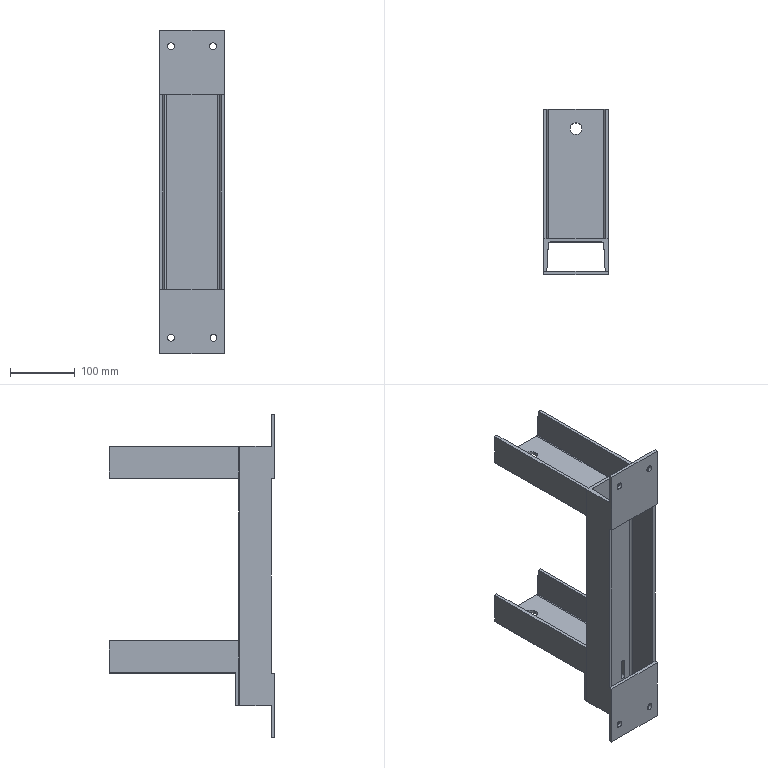Part | SolidWorks | features ICE 5, HoleWzd 2, Extrusion 1 | 1 solid | 74 faces | box 100 x 255 x 500 mm | volume 980990 mm3 | plane 44 | cylinder 30 | commonest cylinder face diameters 2 x10 10.5 x8 8.5 x6 18.5 x4 6 x2